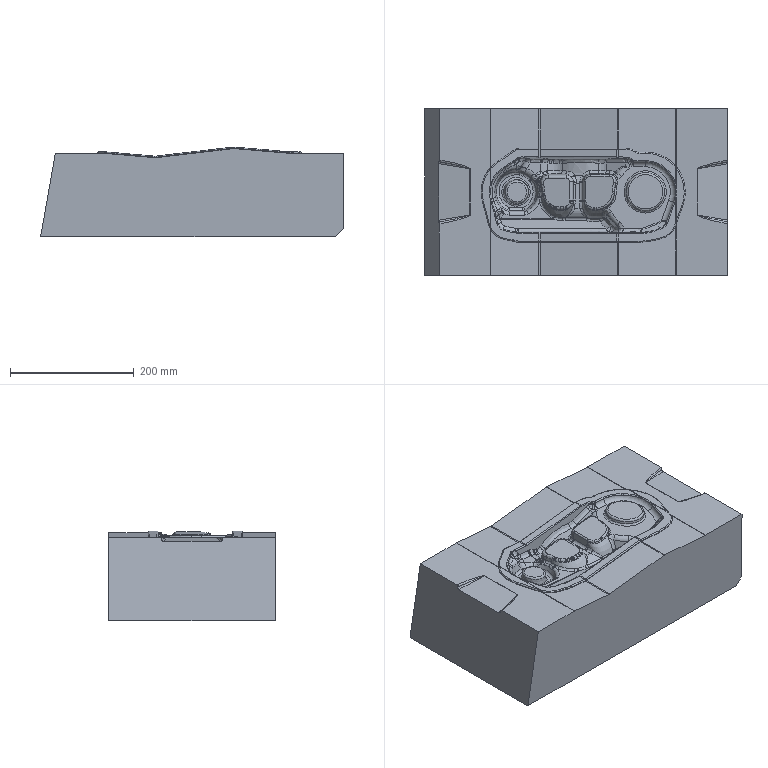NC program | NX | posted with a generic post | part box 490.523 x 270 x 145.452 mm
Lines 1 to 793 of 10809:
N10 G17 G21 G94 G90
(ZLEVEL_PROFILE_1 , TOOL : B8)
N12 T00 M6
N14 G54
N16 G17 G0 G90 X-174.205 Y182.479 S3000 M3
N18 G43 Z100. H0
N20 Z10.073
N22 G94 G1 Z7.073 F2500.
N24 X-174.177 Y184.45
N26 G3 X-176.148 Y186.479 R2.
N28 G2 X-179.03 Y186.577 R72.669
N30 G1 X-179.373 Y186.584 Z7.033
N32 X-179.716 Y186.59 Z6.993
N34 X-180.059 Y186.595 Z6.953
N36 X-180.402 Y186.601 Z6.914
N38 X-180.745 Y186.607 Z6.874
N40 X-180.666 Y186.602
N42 G3 X-173.719 Y186.368 R88.532
N44 G1 X-173.38 Y186.36 Z6.845
N46 X-173.041 Y186.349 Z6.817
N48 X-172.702 Y186.342 Z6.789
N50 X-172.363 Y186.335 Z6.76
N52 X-172.024 Y186.33 Z6.732
N54 X-171.685 Y186.325 Z6.703
N56 X-171.346 Y186.324 Z6.675
N58 X-171.398 Y186.323
N60 G2 X-180.653 Y186.513 R97.153
N62 G1 X-182.419 Y186.634
N64 X-182.763 Y186.639 Z6.635
N66 X-183.107 Z6.595
N68 X-183.452 Y186.64 Z6.556
N70 X-183.796 Z6.516
N72 X-184.141 Z6.476
N74 G3 X-182.744 Y186.57 R243.81
N76 X-170.82 Y186.251 R115.038
N78 X-168.871 Y186.306 R295.102
N80 G1 X-168.543 Y186.305 Z6.448
N82 X-167.559 Y186.299 Z6.363
N84 X-166.903 Y186.295 Z6.306
N86 X-166.575 Y186.292 Z6.277
N88 G2 X-172.355 Y186.14 R409.793
N90 X-182.744 Y186.494 R148.107
N92 X-185.802 Y186.641 R270.998
N94 G1 X-186.143 Y186.642 Z6.238
N96 X-186.484 Z6.198
N98 X-186.824 Z6.158
N100 X-187.165 Y186.641 Z6.118
N102 X-187.506 Y186.638 Z6.079
N104 G3 X-184.822 Y186.513 R243.28
N106 X-173.741 Y186.07 R354.237
N108 X-164.215 Y186.272 R304.981
N110 G1 X-163.875 Y186.279 Z6.045
N112 X-163.534 Y186.275 Z6.012
N114 X-163.193 Y186.272 Z5.979
N116 X-162.852 Y186.268 Z5.946
N118 X-162.512 Y186.265 Z5.913
N120 X-162.171 Y186.258 Z5.88
N122 G3 X-162.486 Y186.253 R4.904
N124 G2 X-175.126 Y186.051 R207.714
N126 G1 X-177.203 Y186.115
N128 X-189.221 Y186.641
N130 X-189.562 Y186.64 Z5.84
N132 X-189.902 Z5.8
N134 X-190.242 Y186.639 Z5.76
N136 X-190.582 Z5.721
N138 X-190.922 Y186.64 Z5.681
N140 G3 X-182.744 Y186.302 R320.167
N142 X-173.048 Y185.969 R367.333
N144 X-162.439 Y186.172 R324.949
N146 G2 X-161.045 Y186.014 R4.742
N148 G1 X-160.765 Y185.908 Z5.631
N150 X-160.489 Y185.778 Z5.582
N152 X-160.221 Y185.629 Z5.532
N154 X-159.968 Y185.459 Z5.482
N156 G3 X-162.403 Y186.089 R4.675
N158 G1 X-170.97 Y185.926
N160 X-172.355 Y185.917
N162 G2 X-180.666 Y186.189 R250.065
N164 X-192.641 Y186.648 R393.716
N166 G1 X-192.982 Y186.637 Z5.442
N168 X-193.323 Z5.403
N170 X-193.664 Z5.363
N172 X-194.005 Y186.636 Z5.323
N174 X-194.345 Y186.637 Z5.283
N176 G3 X-186.207 Y186.31 R313.156
N178 G2 X-175.126 Y185.947 R923.387
N180 G3 X-168.893 Y185.9 R111.624
N182 G1 X-162.66 Y186.018
N184 X-161.967 Y186.014
N186 G2 X-158.897 Y184.457 R4.743
N188 G1 X-158.689 Y184.197 Z5.272
N190 X-158.482 Y183.929 Z5.261
N192 X-158.265 Y183.662 Z5.25
N194 X-158.043 Y183.392 Z5.239
N196 X-157.799 Y183.139 Z5.228
N198 X-157.544 Y182.894 Z5.217
N200 X-157.285 Y182.65 Z5.206
N202 X-157.007 Y182.428 Z5.195
N204 X-156.723 Y182.215 Z5.184
N206 X-156.435 Y182.005 Z5.173
N208 X-156.134 Y181.822 Z5.162
N210 X-155.831 Y181.648 Z5.151
N212 X-155.527 Y181.48 Z5.14
N214 X-155.215 Y181.34 Z5.129
N216 X-154.905 Y181.209 Z5.118
N218 X-154.597 Y181.084 Z5.107
N220 X-154.288 Y180.987 Z5.096
N222 X-153.981 Y180.904 Z5.085
N224 G2 X-158.78 Y184.167 R8.628
N226 G3 X-162.66 Y185.96 R4.512
N228 G2 X-173.741 Y185.873 R324.517
N230 G3 X-186.207 Y186.254 R617.767
N232 G2 X-196.028 Y186.635 R333.029
N234 G1 X-196.373 Y186.629 Z5.045
N236 X-196.717 Y186.628 Z5.005
N238 X-197.062 Y186.627 Z4.965
N240 X-197.407 Z4.925
N242 X-197.751 Y186.634 Z4.886
N244 G3 X-186.207 Y186.214 R336.534
N246 G2 X-173.741 Y185.851 R550.182
N248 G3 X-162.66 Y185.908 R359.156
N250 G2 X-158.885 Y184.167 R4.434
N252 G3 X-158.133 Y183.296 R18.917
N254 X-151.549 Y180.54 R8.538
N256 X-150.146 Y180.591 R445.598
N258 G1 X-149.811 Y180.593 Z4.857
N260 X-149.475 Z4.829
N262 X-149.14 Z4.8
N264 X-148.805 Z4.772
N266 X-148.47 Z4.744
N268 X-148.135 Z4.715
N270 X-147.8 Z4.687
N272 G2 X-151.602 Y180.464 R457.886
N274 X-158.169 Y183.226 R8.581
N276 X-159.081 Y184.283 R21.564
N278 G3 X-162.477 Y185.867 R4.265
N280 G2 X-173.741 Y185.829 R373.284
N282 G3 X-186.207 Y186.179 R447.767
N284 G2 X-199.43 Y186.628 R354.414
N286 G1 X-199.774 Y186.619 Z4.647
N288 X-200.118 Y186.618 Z4.607
N290 X-200.462 Y186.617 Z4.568
N292 X-200.806 Y186.616 Z4.528
N294 X-201.149 Y186.626 Z4.488
N296 G3 X-186.69 Y186.162 R399.838
N298 G1 X-182.744 Y186.106
N300 X-182.051 Y186.094
N302 X-173.741 Y185.807
N304 G3 X-162.66 Y185.822 R377.655
N306 G2 X-159.056 Y184.167 R4.282
N308 G3 X-151.579 Y180.39 R8.912
N310 X-145.454 Y180.594 R523.556
N312 G1 X-145.119 Y180.593 Z4.46
N314 X-144.784 Z4.431
N316 X-144.448 Z4.403
N318 X-144.113 Z4.374
N320 X-143.778 Z4.346
N322 X-143.443 Z4.318
N324 X-143.108 Z4.289
N326 G2 X-151.674 Y180.325 R534.7
N328 X-158.728 Y183.699 R8.642
N330 G3 X-159.521 Y184.597 R8.805
N332 X-162.49 Y185.788 R4.128
N334 G2 X-173.741 Y185.785 R349.176
N336 G1 X-182.051 Y186.074
N338 X-184.129 Y186.107
N340 X-186.207 Y186.131
N342 G2 X-202.873 Y186.622 R415.682
N344 G1 X-203.214 Y186.61 Z4.25
N346 X-203.554 Y186.609 Z4.21
N348 X-203.894 Y186.608 Z4.17
N350 X-204.234 Y186.607 Z4.13
N352 X-204.573 Y186.616 Z4.09
N354 G3 X-185.752 Y186.11 R427.043
N356 G2 X-178.478 Y185.923 R174.223
N358 G3 X-167.822 Y185.714 R197.701
N360 G1 X-162.453 Y185.753
N362 G2 X-159.42 Y184.436 R4.082
N364 X-158.78 Y183.68 R11.818
N366 G3 X-151.634 Y180.27 R8.825
N368 X-140.762 Y180.594 R548.622
N370 G1 X-140.427 Y180.593 Z4.062
N372 X-140.092 Z4.034
N374 X-139.757 Z4.005
N376 X-139.421 Z3.977
N378 X-139.086 Z3.948
N380 X-138.751 Z3.92
N382 X-138.416 Y180.599 Z3.892
N384 G2 X-151.579 Y180.215 R590.007
N386 X-159.118 Y184.015 R9.046
N388 G3 X-162.479 Y185.72 R4.057
N390 G2 X-171.663 Y185.689 R451.202
N392 G1 X-173.741 Y185.741
N394 X-182.051 Y186.035
N396 X-182.744 Y186.049
N398 X-192.44 Y186.162
N400 X-194.517 Y186.202
N402 G2 X-206.319 Y186.615 R418.629
N404 G1 X-206.655 Y186.602 Z3.852
N406 X-206.99 Y186.601 Z3.812
N408 X-207.325 Y186.599 Z3.772
N410 X-207.66 Y186.598 Z3.733
N412 X-207.995 Y186.607 Z3.693
N414 G3 X-192.241 Y186.138 R402.776
N416 G1 X-187.592 Y186.091
N418 X-182.051 Y186.016
N420 X-181.359 Y185.993
N422 X-171.663 Y185.662
N424 G3 X-162.66 Y185.684 R393.187
N426 G2 X-159.197 Y184.073 R4.14
N428 G3 X-151.579 Y180.175 R9.045
N430 X-136.07 Y180.599 R643.806
N432 G1 X-135.735 Y180.593 Z3.664
N434 X-135.4 Z3.636
N436 X-135.065 Z3.608
N438 X-134.729 Z3.579
N440 X-134.394 Z3.551
N442 X-134.059 Z3.522
N444 X-133.724 Y180.594 Z3.494
N446 G2 X-151.579 Y180.147 R662.683
N448 X-159.197 Y184.019 R9.03
N450 G3 X-162.66 Y185.65 R4.125
N452 G2 X-171.663 Y185.634 R373.137
N454 G1 X-173.741 Y185.697
N456 X-182.051 Y185.996
N458 X-184.129 Y186.036
N460 X-195.21 Y186.149
N462 G2 X-209.669 Y186.603 R392.462
N464 G1 X-210.01 Y186.589 Z3.454
N466 X-210.351 Z3.415
N468 X-210.692 Y186.588 Z3.375
N470 X-211.033 Z3.335
N472 X-211.373 Y186.603 Z3.295
N474 G3 X-197.288 Y186.15 R363.435
N476 G1 X-184.129 Y186.019
N478 X-182.744 Y185.994
N480 X-182.051 Y185.977
N482 X-173.048 Y185.653
N484 X-171.663 Y185.607
N486 G3 X-162.542 Y185.618 R329.489
N488 G2 X-160.078 Y184.838 R4.088
N490 X-159.266 Y184.06 R4.133
N492 G1 X-158.804 Y183.475
N494 G3 X-151.579 Y180.12 R8.909
N496 X-132.187 Y180.559 R702.088
N498 G2 X-131.476 Y180.579 R50.288
N500 G1 X-131.173 Y180.563 Z3.267
N502 X-130.869 Y180.556 Z3.238
N504 X-130.565 Y180.548 Z3.21
N506 X-130.262 Y180.532 Z3.182
N508 X-129.958 Y180.512 Z3.153
N510 X-129.655 Y180.492 Z3.125
N512 X-129.351 Y180.483 Z3.096
N514 G3 X-132.879 Y180.46 R50.866
N516 G2 X-151.579 Y180.093 R680.244
N518 X-158.834 Y183.475 R8.894
N520 G1 X-159.197 Y183.93
N522 G3 X-159.394 Y184.171 R4.365
N524 X-162.59 Y185.583 R4.171
N526 G2 X-171.663 Y185.579 R292.026
N528 G1 X-182.051 Y185.957
N530 X-183.436 Y185.991
N532 X-184.822 Y186.011
N534 X-200.058 Y186.159
N536 G2 X-213.089 Y186.599 R327.034
N538 G1 X-213.379 Y186.585 Z3.063
N540 X-213.667 Y186.584 Z3.03
N542 X-213.956 Z2.997
N544 X-214.245 Z2.964
N546 X-214.533 Z2.931
N548 X-214.822 Y186.596 Z2.898
N550 G3 X-204.906 Y186.215 R316.501
N552 X-184.129 Y185.985 R2559.071
N554 G1 X-182.051 Y185.938
N556 X-171.663 Y185.552
N558 G3 X-162.66 Y185.548 R305.078
N560 G2 X-159.197 Y183.886 R4.156
N562 G3 X-151.579 Y180.065 R8.999
N564 X-132.433 Y180.397 R851.522
N566 G2 X-127.269 Y180.281 R50.536
N568 G1 X-126.966 Y180.245 Z2.869
N570 X-126.664 Y180.208 Z2.841
N572 X-126.362 Y180.163 Z2.812
N574 X-126.06 Y180.118 Z2.784
N576 X-125.758 Y180.073 Z2.756
N578 X-125.457 Y180.028 Z2.727
N580 X-125.155 Y179.981 Z2.699
N582 G3 X-132.187 Y180.338 R50.038
N584 G2 X-151.579 Y180.038 R1040.339
N586 X-159.197 Y183.838 R8.969
N588 G3 X-162.66 Y185.513 R4.143
N590 G2 X-177.896 Y185.763 R232.605
N592 G3 X-189.67 Y186.027 R274.25
N594 G2 X-206.291 Y186.212 R1352.365
N596 X-216.505 Y186.59 R309.982
N598 G1 X-216.84 Y186.579 Z2.659
N600 X-217.174 Y186.578 Z2.619
N602 X-217.508 Y186.577 Z2.58
N604 X-217.842 Y186.576 Z2.54
N606 X-218.176 Y186.589 Z2.5
N608 G3 X-206.984 Y186.18 R315.302
N610 X-188.284 Y185.999 R2509.179
N612 G2 X-177.896 Y185.743 R249.725
N614 G3 X-162.66 Y185.479 R242.656
N616 G2 X-159.197 Y183.786 R4.119
N618 G3 X-152.162 Y180.017 R8.874
N620 X-132.187 Y180.282 R1235.655
N622 G2 X-123.115 Y179.591 R49.774
N624 G1 X-122.811 Y179.526 Z2.473
N626 X-122.507 Y179.456 Z2.445
N628 X-122.204 Y179.386 Z2.418
N630 X-121.901 Y179.315 Z2.39
N632 X-121.597 Y179.244 Z2.363
N634 X-121.295 Y179.172 Z2.335
N636 X-120.992 Y179.096 Z2.308
N638 G3 X-132.187 Y180.224 R48.968
N640 G1 X-132.879 Y180.212
N642 X-141.19 Y180.092
N644 X-141.883 Y180.097
N646 G3 X-151.579 Y179.953 R451.749
N648 G2 X-159.197 Y183.726 R8.938
N650 G3 X-162.66 Y185.444 R4.085
N652 G2 X-177.896 Y185.722 R251.009
N654 G3 X-188.284 Y185.983 R250.922
N656 G1 X-205.598 Y186.127
N658 X-207.676 Y186.154
N660 G2 X-219.868 Y186.582 R309.457
N662 G1 X-220.204 Y186.574 Z2.269
N664 X-220.54 Z2.231
N666 X-220.876 Z2.192
N668 X-221.211 Z2.154
N670 X-221.547 Y186.572 Z2.115
N672 G3 X-211.139 Y186.188 R273.286
N674 X-188.284 Y185.968 R2380.24
N676 G2 X-177.896 Y185.702 R252.085
N678 G3 X-162.66 Y185.41 R259.609
N680 G2 X-159.197 Y183.669 R4.089
N682 G3 X-151.604 Y179.901 R8.87
N684 G2 X-148.391 Y179.981 R127.404
N686 G1 X-132.187 Y180.18
N688 G2 X-118.988 Y178.517 R48.66
N690 G1 X-118.696 Y178.411 Z2.088
N692 X-118.401 Y178.316 Z2.06
N694 X-118.106 Y178.221 Z2.033
N696 X-117.81 Y178.126 Z2.005
N698 X-117.519 Y178.02 Z1.978
N700 X-117.227 Y177.912 Z1.951
N702 X-116.933 Y177.815 Z1.923
N704 G3 X-132.879 Y180.14 R48.545
N706 G1 X-145.278 Y180.001
N708 G3 X-151.654 Y179.848 R250.982
N710 G2 X-159.197 Y183.592 R8.826
N712 G3 X-162.66 Y185.375 R4.107
N714 G2 X-177.101 Y185.65 R249.89
N716 G3 X-188.112 Y185.954 R270.98
N718 G1 X-206.984 Y186.092
N720 X-208.369 Y186.11
N722 G2 X-223.177 Y186.581 R330.456
N724 G1 X-223.511 Y186.57 Z1.885
N726 X-223.845 Y186.569 Z1.846
N728 X-224.178 Z1.808
N730 X-224.512 Z1.769
N732 X-224.845 Y186.582 Z1.731
N734 G3 X-209.754 Y186.101 R332.812
N736 G1 X-207.676 Y186.074
N738 X-190.362 Y185.955
N740 G2 X-177.203 Y185.634 R302.378
N742 G3 X-162.66 Y185.317 R293.633
N744 G2 X-159.197 Y183.502 R4.067
N746 G3 X-151.579 Y179.788 R8.752
N748 G2 X-132.879 Y180.108 R683.882
N750 G1 X-132.187 Y180.126
N752 G2 X-114.842 Y176.983 R48.483
N754 G1 Z3.731
N756 G0 Z4.923
N758 X-154.606 Y175.944
N760 Z4.538
N762 G1 Z1.538
N764 X-153.951 Y177.659
N766 G3 X-155.105 Y180.241 R2.
N768 G2 X-156.624 Y181.009 R8.247
N770 G1 X-156.872 Y181.168
N772 G2 X-159.302 Y183.529 R8.562
N774 G3 X-162.66 Y185.259 R3.981
N776 G2 X-177.203 Y185.614 R357.767
N778 G3 X-190.362 Y185.94 R308.21
N780 G1 X-209.754 Y186.073
N782 X-214.547 Y186.151
N784 G2 X-226.497 Y186.576 R309.35
N786 G1 X-226.823 Y186.568 Z1.5
N788 X-227.148 Z1.462
N790 X-227.473 Z1.423
N792 X-227.798 Z1.385
N794 X-228.123 Y186.574 Z1.346
N796 G3 X-211.139 Y186.065 R383.814
N798 G1 X-188.284 Y185.906
N800 X-184.822 Y185.861
N802 X-183.436 Y185.829
N804 X-171.663 Y185.382
N806 G3 X-162.525 Y185.198 R686.125
N808 G2 X-159.72 Y183.892 R3.775
N810 G1 X-159.628 Y183.785
N812 X-159.823 Y184.015 Z1.329
N814 X-160.06 Y184.233 Z1.311
N816 X-160.329 Y184.438 Z1.294
N818 X-160.63 Y184.622 Z1.276
N820 X-160.955 Y184.779 Z1.259
N822 X-161.292 Y184.916 Z1.241
N824 X-161.642 Y185.017 Z1.224
N826 X-161.996 Y185.081 Z1.206
N828 X-162.345 Y185.109 Z1.189
N830 X-162.679 Y185.127 Z1.171
N832 X-162.998 Y185.13 Z1.154
N834 G3 X-169.585 Y185.293 R223.415
N836 G1 X-171.663 Y185.361
N838 X-183.436 Y185.81
N840 X-184.822 Y185.842
N842 X-188.284 Y185.891
N844 X-213.217 Y186.064
N846 G2 X-229.844 Y186.588 R364.841
N848 G1 X-230.161 Y186.573 Z1.115
N850 X-230.477 Y186.572 Z1.077
N852 X-230.793 Z1.038
N854 X-231.109 Y186.571 Z1.
N856 X-231.425 Y186.58 Z0.962
N858 G3 X-212.524 Y186.04 R374.604
N860 G1 X-188.284 Y185.875
N862 X-184.822 Y185.824
N864 X-183.436 Y185.79
N866 X-169.585 Y185.268
N868 X-168.893 Y185.249
N870 X-167.077 Y185.209
N872 G2 X-163.916 Y185.09 R98.395
N874 G1 X-164.185 Y185.075 Z0.897
N876 X-164.455 Y185.063 Z0.833
N878 X-164.724 Y185.047 Z0.769
N880 G3 X-167.538 Y185.181 R81.375
N882 G1 X-169.585 Y185.243
N884 X-183.436 Y185.771
N886 X-184.822 Y185.806
N888 X-188.977 Y185.866
N890 X-215.288 Y186.041
N892 G2 X-233.101 Y186.584 R373.906
N894 G1 X-233.426 Y186.574 Z0.731
N896 X-233.752 Z0.692
N898 X-234.077 Z0.654
N900 X-234.402 Z0.615
N902 X-234.727 Y186.572 Z0.577
N904 G3 X-215.905 Y186.028 R423.166
N906 G1 X-188.284 Y185.843
N908 X-184.822 Y185.788
N910 X-183.436 Y185.751
N912 X-169.585 Y185.218
N914 X-168.893 Y185.195
N916 G2 X-165.346 Y185.009 R63.475
N918 G1 X-165.641 Y184.995 Z0.481
N920 X-165.937 Y184.971 Z0.385
N922 G3 X-167.508 Y185.118 R90.242
N924 G1 X-183.436 Y185.732
N926 X-184.822 Y185.77
N928 G3 X-207.676 Y185.952 R2086.1
N930 G2 X-226.1 Y186.175 R931.664
N932 X-236.403 Y186.581 R296.164
N934 G1 X-236.728 Y186.576 Z0.346
N936 X-237.053 Z0.308
N938 X-237.379 Z0.269
N940 X-237.704 Z0.231
N942 X-238.028 Y186.583 Z0.192
N944 G3 X-227.76 Y186.169 R300.134
N946 X-208.369 Y185.938 R1220.444
N948 G2 X-184.822 Y185.752 R2069.915
N950 G1 X-183.436 Y185.712
N952 X-168.2 Y185.116
N954 G2 X-166.461 Y184.932 R69.919
N956 G1 X-166.694 Z0.096
N958 X-166.93 Y184.91 Z0.
N960 G3 X-168.2 Y185.063 R51.032
N962 G1 X-168.893 Y185.111
N964 X-183.436 Y185.694
N966 X-186.207 Y185.766
N968 X-189.67 Y185.811
N970 X-217.247 Y185.983
N972 G2 X-233.893 Y186.314 R611.32
N974 X-239.642 Y186.574 R244.574
N976 G1 X-239.937 Y186.576 Z-0.033
N978 X-240.232 Y186.577 Z-0.067
N980 X-240.527 Y186.578 Z-0.1
N982 X-240.822 Z-0.133
N984 X-241.117 Y186.579 Z-0.167
N986 X-241.412 Y186.578 Z-0.2
N988 G3 X-231.916 Y186.198 R257.479
N990 X-212.524 Y185.932 R958.795
N992 G1 X-189.67 Y185.794
N994 X-186.207 Y185.747
N996 X-183.436 Y185.673
N998 X-171.663 Y185.213
N1000 X-169.585 Y185.113
N1002 G2 X-167.445 Y184.884 R31.262
N1004 G1 X-167.686 Y184.887 Z-0.3
N1006 X-167.93 Y184.868 Z-0.4
N1008 G3 X-170.278 Y185.123 R24.627
N1010 G1 X-171.663 Y185.189
N1012 X-183.436 Y185.652
N1014 X-186.207 Y185.73
N1016 X-191.055 Y185.791
N1018 X-213.217 Y185.919
N1020 G2 X-235.361 Y186.241 R1006.353
N1022 X-243.152 Y186.582 R260.007
N1024 G1 X-243.489 Y186.589 Z-0.44
N1026 X-243.827 Z-0.48
N1028 X-244.164 Y186.59 Z-0.52
N1030 X-244.502 Y186.591 Z-0.56
N1032 X-244.839 Y186.596 Z-0.6
N1034 G3 X-237.034 Y186.241 R282.677
N1036 G1 X-231.916 Y186.117
N1038 X-229.838 Y186.068
N1040 X-213.217 Y185.9
N1042 X-191.055 Y185.775
N1044 X-187.592 Y185.736
N1046 G2 X-170.597 Y185.098 R625.694
N1048 X-168.4 Y184.858 R19.147
N1050 G1 X-168.645 Y184.851 Z-0.7
N1052 X-168.889 Y184.844 Z-0.8
N1054 G3 X-171.25 Y185.113 R22.634
N1056 G1 X-171.663 Y185.138
N1058 X-184.822 Y185.658
N1060 X-187.592 Y185.719
N1062 X-191.055 Y185.759
N1064 X-212.524 Y185.877
N1066 X-230.501 Y186.062
N1068 G2 X-246.577 Y186.608 R340.777
N1070 G1 X-246.919 Y186.599 Z-0.84
N1072 X-247.26 Y186.6 Z-0.88
N1074 X-247.601 Y186.601 Z-0.92
N1076 X-247.942 Y186.602 Z-0.96
N1078 X-248.282 Y186.617 Z-1.
N1080 G3 X-232.608 Y186.061 R358.959
N1082 G1 X-212.524 Y185.859
N1084 X-191.055 Y185.743
N1086 X-187.592 Y185.703
N1088 X-184.822 Y185.639
N1090 X-172.355 Y185.146
N1092 X-171.663 Y185.11
N1094 G2 X-169.39 Y184.833 R21.101
N1096 G1 X-169.638 Y184.836 Z-1.1
N1098 X-169.888 Y184.831 Z-1.2
N1100 G3 X-172.355 Y185.121 R18.043
N1102 G1 X-184.822 Y185.62
N1104 X-187.592 Y185.686
N1106 X-191.055 Y185.727
N1108 X-212.524 Y185.841
N1110 X-213.909 Y185.849
N1112 X-234.686 Y186.067
N1114 X-235.379 Y186.083
N1116 X-239.482 Y186.184
N1118 G2 X-250.002 Y186.617 R323.25
N1120 G1 X-250.292 Y186.61 Z-1.233
N1122 X-250.582 Y186.611 Z-1.267
N1124 X-250.872 Y186.612 Z-1.3
N1126 X-251.162 Y186.614 Z-1.333
N1128 X-251.451 Y186.615 Z-1.367
N1130 X-251.74 Y186.627 Z-1.4
N1132 G3 X-241.612 Y186.196 R318.898
N1134 X-218.065 Y185.864 R1298.964
N1136 G1 X-191.055 Y185.711
N1138 X-189.67 Y185.697
N1140 G2 X-172.355 Y185.081 R456.11
N1142 X-170.387 Y184.831 R16.563
N1144 G1 X-170.645 Z-1.5
N1146 X-170.904 Y184.829 Z-1.6
N1148 G3 X-173.741 Y185.137 R21.598
N1150 G1 X-184.822 Y185.583
N1152 X-187.592 Y185.652
N1154 G3 X-213.909 Y185.812 R4115.588
N1156 G1 X-218.065 Y185.845
N1158 X-238.149 Y186.073
N1160 X-240.227 Y186.118
N1162 G2 X-253.427 Y186.633 R351.939
N1164 G1 X-253.718 Y186.621 Z-1.633
N1166 X-254.007 Y186.622 Z-1.667
N1168 X-254.297 Y186.623 Z-1.7
N1170 X-254.587 Y186.624 Z-1.733
N1172 X-254.877 Y186.625 Z-1.767
N1174 X-255.165 Y186.642 Z-1.8
N1176 G3 X-242.304 Y186.13 R353.101
N1178 G1 X-241.612 Y186.122
N1180 X-240.919 Y186.105
N1182 X-239.534 Y186.07
N1184 X-218.065 Y185.826
N1186 X-213.909 Y185.794
N1188 G2 X-187.592 Y185.636 R3889.08
N1190 G1 X-186.207 Y185.606
N1192 X-174.433 Y185.145
N1194 X-173.741 Y185.109
N1196 G2 X-171.408 Y184.823 R18.826
N1198 G1 X-171.66 Y184.829 Z-1.9
N1200 X-171.914 Y184.826 Z-2.
N1202 G3 X-174.797 Y185.129 R27.792
N1204 X-197.288 Y185.708 R419.206
N1206 G2 X-241.612 Y186.085 R3225.983
N1208 X-256.853 Y186.639 R411.638
N1210 G1 X-257.143 Y186.631 Z-2.033
N1212 X-257.433 Y186.633 Z-2.067
N1214 X-257.722 Y186.634 Z-2.1
N1216 X-258.012 Y186.635 Z-2.133
N1218 X-258.302 Y186.636 Z-2.167
N1220 X-258.591 Y186.651 Z-2.2
N1222 G3 X-242.304 Y186.067 R406.647
N1224 X-196.595 Y185.69 R3381.031
N1226 G2 X-174.433 Y185.081 R404.459
N1228 X-172.427 Y184.828 R17.427
N1230 G1 X-172.683 Y184.829 Z-2.3
N1232 X-172.941 Y184.824 Z-2.4
N1234 G3 X-175.318 Y185.105 R18.374
N1236 X-189.67 Y185.616 R416.752
N1238 G1 X-193.825 Y185.654
N1240 X-208.689 Y185.717
N1242 G2 X-246.115 Y186.116 R2913.794
N1244 X-260.328 Y186.657 R339.198
N1246 G1 X-260.666 Y186.645 Z-2.44
N1248 X-261.004 Z-2.48
N1250 X-261.341 Y186.646 Z-2.52
N1252 X-261.679 Y186.647 Z-2.56
N1254 X-262.016 Y186.657 Z-2.6
N1256 G3 X-249.922 Y186.164 R311.016
N1258 X-197.98 Y185.663 R2923.099
N1260 G2 X-176.245 Y185.131 R406.273
N1262 X-173.445 Y184.819 R23.597
N1264 G1 X-173.692 Y184.826 Z-2.7
N1266 X-173.941 Y184.823 Z-2.8
N1268 G3 X-176.114 Y185.084 R16.887
N1270 X-196.595 Y185.642 R368.88
N1272 G2 X-250.615 Y186.146 R3207.242
N1274 X-263.802 Y186.665 R327.35
N1276 G1 X-264.13 Y186.658 Z-2.84
N1278 X-264.458 Z-2.88
N1280 X-264.786 Z-2.92
N1282 X-265.114 Z-2.96
N1284 X-265.441 Y186.665 Z-3.
N1286 G3 X-252.693 Y186.157 R315.316
N1288 X-196.595 Y185.626 R3279.378
N1290 G2 X-176.511 Y185.082 R368.641
N1292 X-174.432 Y184.819 R16.924
N1294 G1 X-174.7 Y184.822 Z-3.1
N1296 X-174.97 Y184.82 Z-3.2
N1298 G3 X-177.203 Y185.096 R20.02
N1300 X-196.595 Y185.61 R359.654
N1302 G2 X-252. Y186.12 R3332.991
N1304 X-267.179 Y186.672 R342.549
N1306 G1 X-267.469 Y186.666 Z-3.233
N1308 X-267.759 Y186.668 Z-3.267
N1310 X-268.049 Y186.669 Z-3.3
N1312 X-268.338 Y186.67 Z-3.333
N1314 X-268.628 Y186.671 Z-3.367
N1316 X-268.917 Y186.678 Z-3.4
N1318 G3 X-254.77 Y186.142 R341.732
N1320 X-196.595 Y185.595 R3427.421
N1322 G2 X-178.317 Y185.132 R359.65
N1324 X-175.481 Y184.817 R23.922
N1326 G1 X-175.732 Y184.824 Z-3.5
N1328 X-175.985 Y184.816 Z-3.6
N1330 G3 X-178.589 Y185.121 R19.613
N1332 X-196.595 Y185.579 R356.458
N1334 G2 X-256.637 Y186.153 R3436.987
N1336 X-270.604 Y186.685 R354.652
N1338 G1 X-270.951 Y186.677 Z-3.64
N1340 X-271.296 Y186.678 Z-3.68
N1342 X-271.642 Y186.68 Z-3.72
N1344 X-271.988 Y186.681 Z-3.76
N1346 X-272.333 Y186.687 Z-3.8
N1348 G3 X-258.988 Y186.177 R346.726
N1350 X-196.595 Y185.563 R3427.599
N1352 G2 X-178.589 Y185.083 R327.955
N1354 X-176.495 Y184.822 R17.118
N1356 G1 X-176.751 Y184.823 Z-3.9
N1358 X-177.008 Y184.817 Z-4.
N1360 G3 X-179.281 Y185.097 R18.526
N1362 X-196.595 Y185.547 R326.125
N1364 G2 X-259.652 Y186.163 R3474.298
N1366 X-274.052 Y186.698 R394.612
N1368 G1 Z-2.
N1370 G0 Z-0.8
N1372 X-277.961 Y182.802
N1374 Z-1.2
N1376 G1 Z-4.2
N1378 X-277.857 Y184.792
N1380 G2 X-275.755 Y186.685 R2.
N1382 G3 X-258.672 Y186.113 R456.654
N1384 G1 X-253.385 Y186.035
N1386 G3 X-197.98 Y185.536 R3263.797
N1388 G2 X-180.666 Y185.146 R343.425
N1390 X-177.519 Y184.818 R22.197
N1392 G1 X-177.772 Y184.823 Z-4.3
N1394 X-178.027 Y184.816 Z-4.4
N1396 G3 X-180.666 Y185.122 R19.615
N1398 X-197.98 Y185.52 R338.78
N1400 G2 X-253.385 Y186.017 R3178.492
N1402 G1 X-260.606 Y186.128
N1404 G2 X-276.528 Y186.635 R481.732
N1406 X-277.469 Y186.682 R224.094
N1408 G1 X-277.815 Y186.688 Z-4.44
N1410 X-278.161 Z-4.48
N1412 X-278.507 Y186.689 Z-4.52
N1414 X-278.852 Z-4.56
N1416 X-279.198 Y186.688 Z-4.6
N1418 G3 X-270.007 Y186.313 R286.022
N1420 X-252. Y185.98 R913.305
N1422 X-197.825 Y185.509 R2964.292
N1424 G2 X-181.189 Y185.123 R351.314
N1426 X-178.527 Y184.817 R19.875
N1428 G1 X-178.781 Y184.821 Z-4.7
N1430 X-179.038 Y184.811 Z-4.8
N1432 G3 X-182.051 Y185.138 R19.814
N1434 X-199.06 Y185.501 R362.887
N1436 G2 X-235.725 Y185.727 R2219.78
N1438 G1 X-265.851 Y186.162
N1440 X-267.929 Y186.21
N1442 G2 X-280.914 Y186.706 R357.177
N1444 G1 X-281.253 Y186.692 Z-4.84
N1446 X-281.592 Z-4.88
N1448 X-281.93 Z-4.92
N1450 X-282.268 Z-4.96
N1452 X-282.607 Y186.699 Z-5.
N1454 G3 X-271.327 Y186.255 R337.788
N1456 G1 X-267.237 Y186.163
N1458 X-235.175 Y185.702
N1460 G3 X-199.129 Y185.485 R2161.872
N1462 G2 X-182.744 Y185.146 R355.757
N1464 X-179.549 Y184.815 R22.505
N1466 G1 X-179.804 Y184.82 Z-5.1
N1468 X-180.06 Y184.818 Z-5.2
N1470 G3 X-183.562 Y185.167 R29.681
N1472 X-198.423 Y185.46 R368.716
N1474 G2 X-254.77 Y185.969 R2992.413
N1476 X-274.855 Y186.318 R1323.212
N1478 X-284.336 Y186.686 R271.824
N1480 G1 X-284.682 Y186.696 Z-5.24
N1482 X-285.027 Z-5.28
N1484 X-285.373 Y186.697 Z-5.32
N1486 X-285.719 Z-5.36
N1488 X-286.064 Y186.707 Z-5.4
N1490 G3 X-273.893 Y186.241 R331.77
N1492 G1 X-272.777 Y186.223
N1494 X-270.007 Y186.165
N1496 X-252. Y185.909
N1498 X-241.424 Y185.741
N1500 G3 X-199.184 Y185.453 R2346.881
N1502 G2 X-183.436 Y185.13 R347.08
N1504 X-180.572 Y184.816 R20.049
N1506 G1 X-180.827 Y184.82 Z-5.5
N1508 X-181.085 Y184.811 Z-5.6
N1510 G3 X-184.129 Y185.138 R19.982
N1512 X-199.349 Y185.437 R340.989
N1514 G2 X-236.907 Y185.665 R2145.314
N1516 G1 X-272.777 Y186.197
N1518 X-274.162 Y186.221
N1520 G2 X-287.755 Y186.7 R335.043
N1522 G1 X-288.1 Y186.698 Z-5.64
N1524 X-288.444 Y186.697 Z-5.68
N1526 X-288.788 Y186.696 Z-5.72
N1528 X-289.132 Z-5.76
N1530 X-289.476 Y186.7 Z-5.8
N1532 G3 X-275.6 Y186.22 R349.15
N1534 G1 X-235.812 Y185.635
N1536 G3 X-199.444 Y185.421 R2059.382
N1538 G2 X-184.822 Y185.146 R335.908
N1540 X-181.579 Y184.807 R20.63
N1542 G1 X-181.814 Y184.814 Z-5.9
N1544 X-182.053 Y184.8 Z-6.
N1546 G3 X-185.232 Y185.148 R22.691
N1548 X-199.5 Y185.405 R346.877
N1550 G2 X-242.89 Y185.705 R2283.366
N1552 G1 X-252. Y185.855
N1554 X-276.932 Y186.217
N1556 G2 X-291.175 Y186.701 R358.112
N1558 G1 X-291.517 Y186.69 Z-6.04
N1560 X-291.858 Z-6.08
N1562 X-292.199 Y186.689 Z-6.12
N1564 X-292.541 Y186.688 Z-6.16
N1566 X-292.881 Y186.695 Z-6.2
N1568 G3 X-278.95 Y186.224 R357.192
N1570 G1 X-252. Y185.837
N1572 X-243.184 Y185.69
N1574 G3 X-200.356 Y185.39 R2225.805
N1576 G2 X-185.971 Y185.161 R387.564
N1578 X-182.595 Y184.807 R24.267
N1580 G1 X-182.854 Y184.817 Z-6.3
N1582 X-183.115 Y184.808 Z-6.4
N1584 G3 X-186.795 Y185.175 R27.192